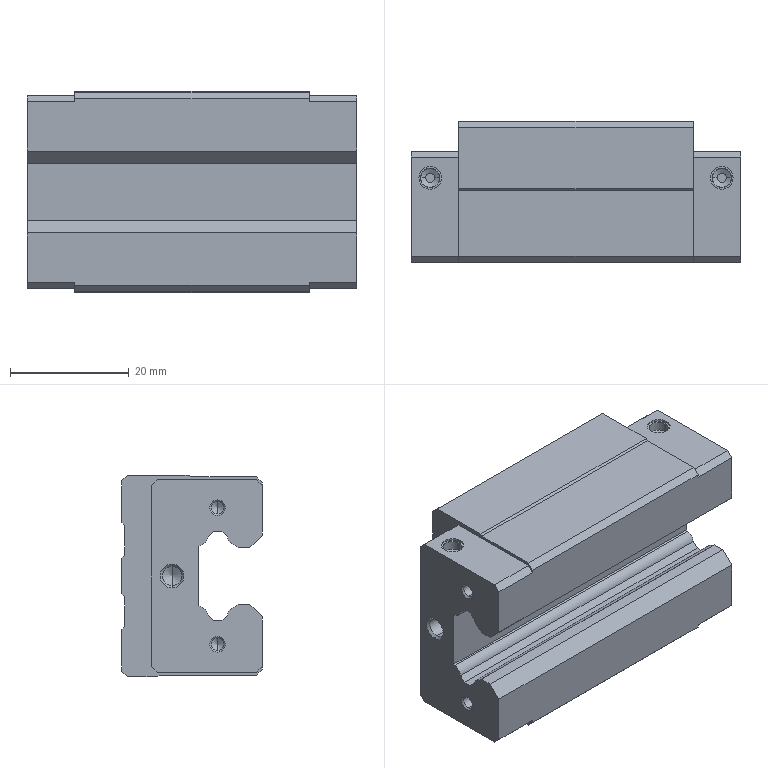Part | STEP file | Block_HGH15CAZ0C | 1 solid | 158 faces | box 55.4 x 23.7 x 34 mm | volume 33117 mm3 | plane 62 | cone 56 | cylinder 40 | commonest cylinder face diameters 3.242 x12 2.113 x8 3.14 x8 3.8 x8 3.2 x4